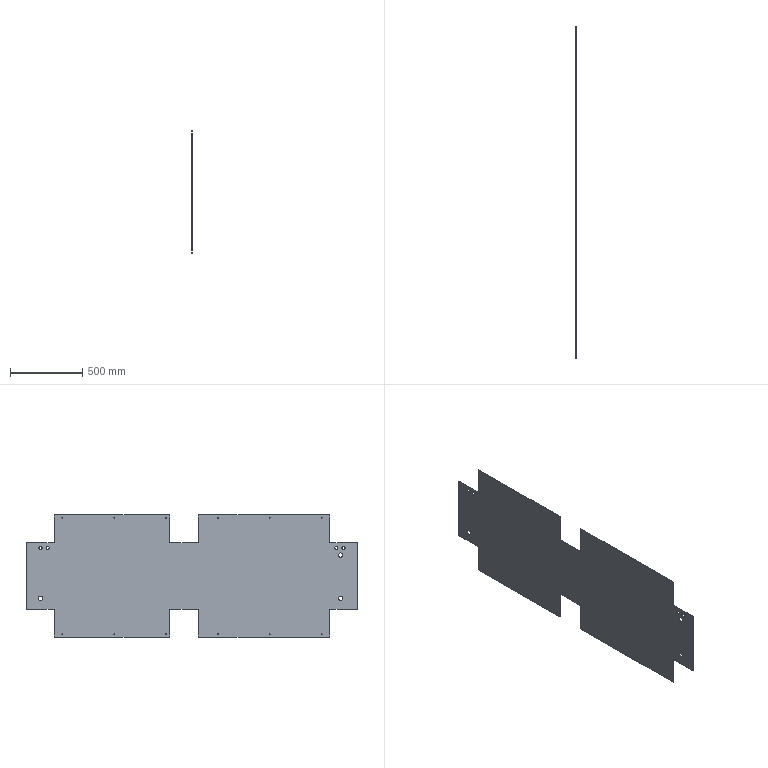Part | NX | 1 solid | 72 faces | box 2 x 2300 x 850 mm | volume 3441418 mm3 | cylinder 50 | plane 22 | commonest cylinder face diameters 6.5 x24 4 x12 23 x8 30 x6